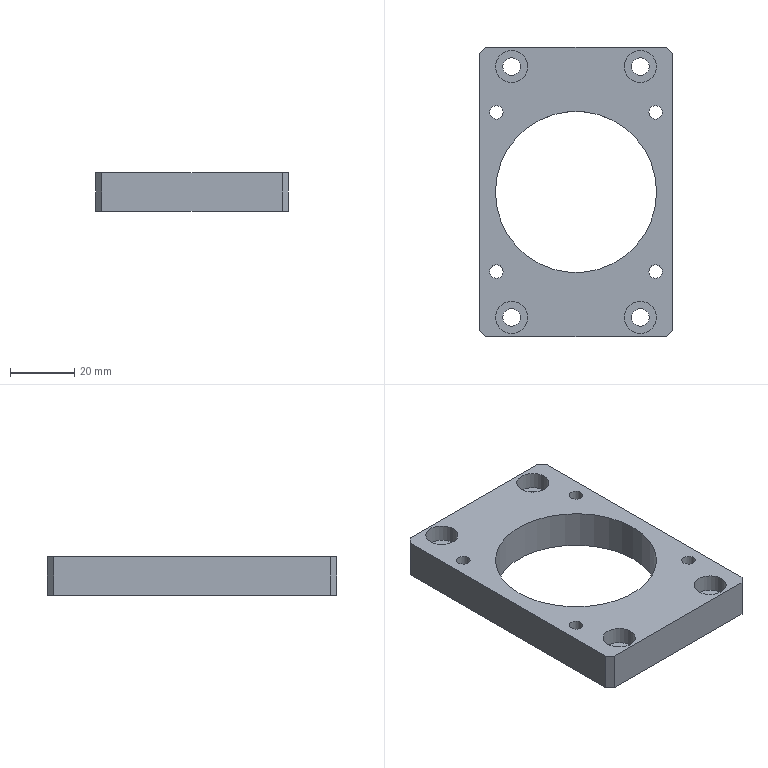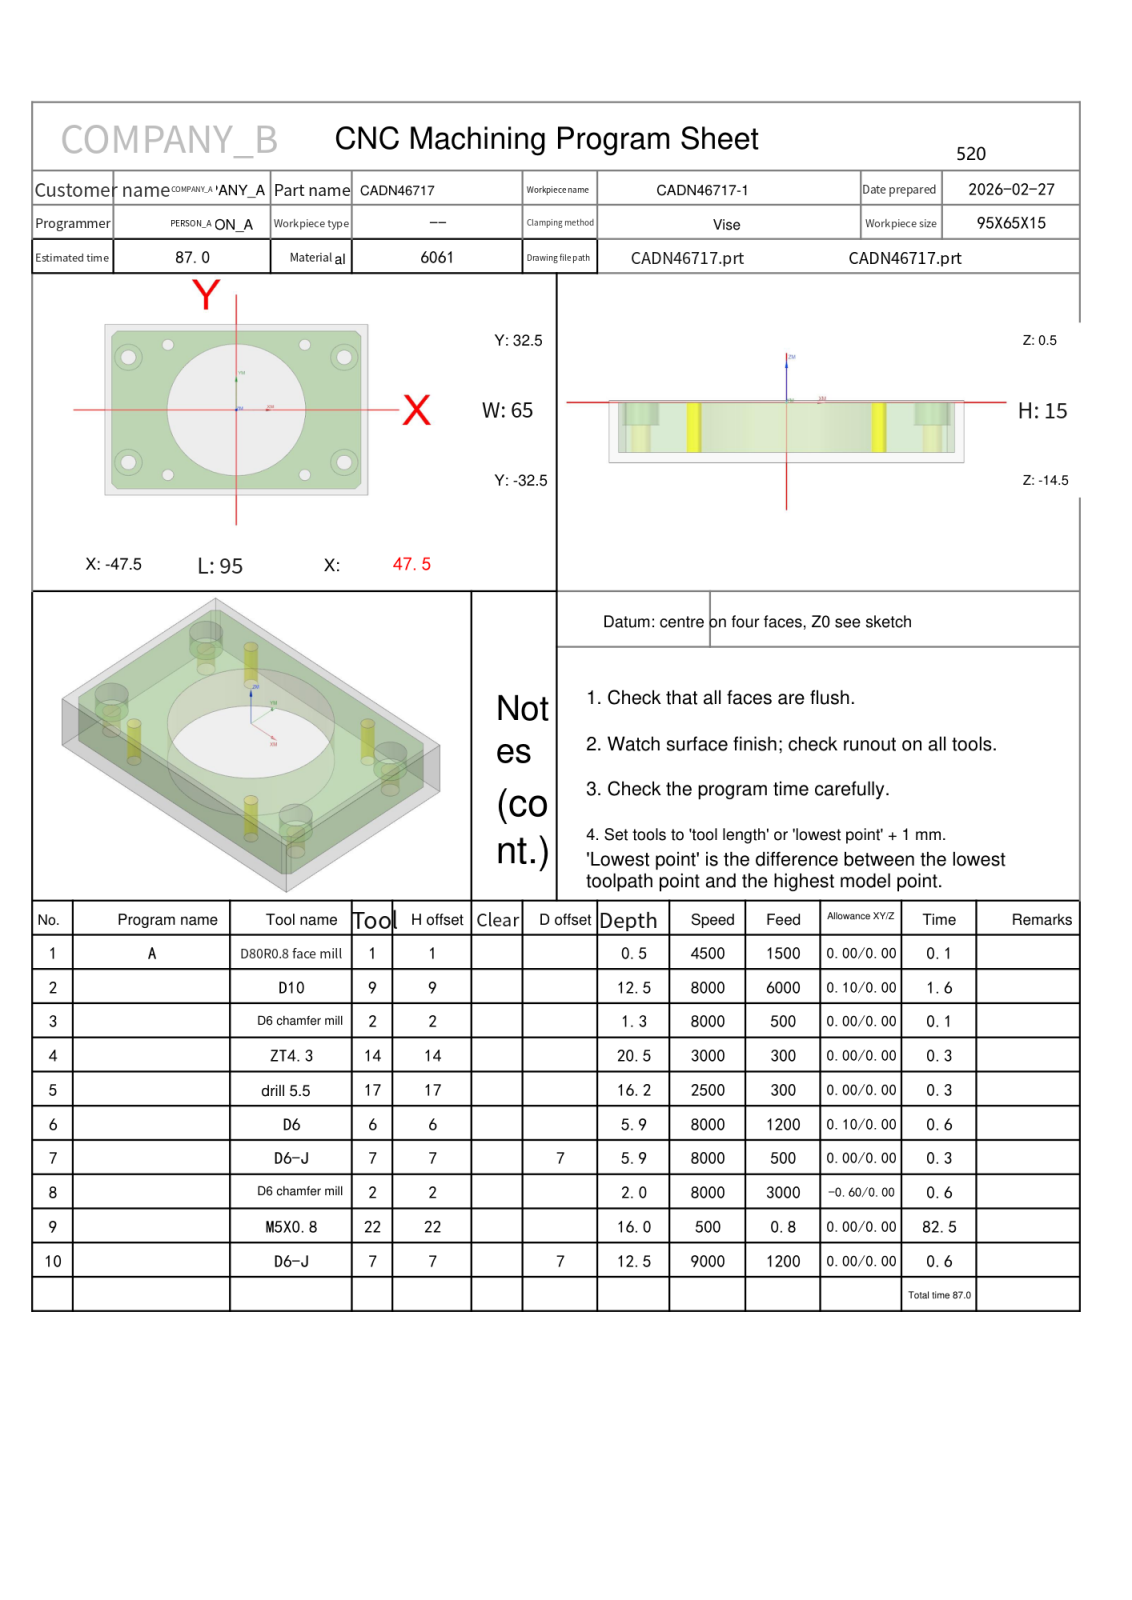NC program | NX | posted by the shop | part box 60 x 90 x 12 mm
Whole program:
%
O0001
(Machine time: 166.41 MIN)
(===Total Tool:8===)
(T1=D80R0.8 face mill D=80.  R=0.8  D-  H01 Z=-0.   )
(T9=D10     D=10.  R=0.   D-  H09 Z=-12.  )
(T2=D6 chamfer mill   D=6.   R=0.   D-  H02 Z=-1.5  )
(T14=ZT4.3  D=4.3  DR_a=118 D-  H14 Z=-20.  )
(T17=drill 5.5  D=5.5  DR_a=118 D-  H17 Z=-15.65)
(T6=D6      D=6.   R=0.   D-  H06 Z=-5.4  )
(T7=D6-J    D=6.   R=0.   D7  H07 Z=-12.  )
(T22=M5X0.8 D=4.2  DR_a=180 D-  H22 Z=-15.5 )
G80 G90 G17 G49 G40
G91 G28 Z0
M01
N1 T01 M06
(D80R0.8 face mill  D=80. R=0.8 H=01 ce=0.00 di=0.00)
G00 G90 G54 X-90. Y0.0 M03 S4500
G43 H01 Z50.
M08
Z2.
G01 Z0.0 F1500.
X-85.
X85.
X90.
Z2.
G00 Z50.
G91 G28 Z0.0
M05
M09
G91 G28 Z0.0
M01
N2 T09 M06
(D10  D=10. R=0. H=09 ce=0.10 di=0.00)
G00 G90 G54 X0.0 Y35.1 M03 S8000
G43 H09 Z50.
M08
Z.5
G01 X43. Z.397 F6000.
G02 X46.606 Y33.606 Z.388 I0.0 J-5.1
G01 X48.606 Y31.606 Z.381
G02 X50.1 Y28. Z.372 I-3.606 J-3.606
G01 Y-28. Z.238
G02 X48.606 Y-31.606 Z.228 I-5.1 J0.0
G01 X46.606 Y-33.606 Z.222
G02 X43. Y-35.1 Z.212 I-3.606 J3.606
G01 X-43. Z.007
G02 X-46.606 Y-33.606 Z-.003 I0.0 J5.1
G01 X-48.606 Y-31.606 Z-.01
G02 X-50.1 Y-28. Z-.019 I3.606 J3.606
G01 Y28. Z-.153
G02 X-48.606 Y31.606 Z-.162 I5.1 J0.0
G01 X-46.606 Y33.606 Z-.169
G02 X-43. Y35.1 Z-.179 I3.606 J-3.606
G01 X43. Z-.384
G02 X46.606 Y33.606 Z-.393 I0.0 J-5.1
G01 X48.606 Y31.606 Z-.4
G02 X50.1 Y28. Z-.41 I-3.606 J-3.606
G01 Y-28. Z-.543
G02 X48.606 Y-31.606 Z-.553 I-5.1 J0.0
G01 X46.606 Y-33.606 Z-.56
G02 X43. Y-35.1 Z-.569 I-3.606 J3.606
G01 X-43. Z-.774
G02 X-46.606 Y-33.606 Z-.784 I0.0 J5.1
G01 X-48.606 Y-31.606 Z-.791
G02 X-50.1 Y-28. Z-.8 I3.606 J3.606
G01 Y28. Z-.934
G02 X-48.606 Y31.606 Z-.944 I5.1 J0.0
G01 X-46.606 Y33.606 Z-.95
G02 X-43. Y35.1 Z-.96 I3.606 J-3.606
G01 X43. Z-1.165
G02 X46.606 Y33.606 Z-1.175 I0.0 J-5.1
G01 X48.606 Y31.606 Z-1.181
G02 X50.1 Y28. Z-1.191 I-3.606 J-3.606
G01 Y-28. Z-1.325
G02 X48.606 Y-31.606 Z-1.334 I-5.1 J0.0
G01 X46.606 Y-33.606 Z-1.341
G02 X43. Y-35.1 Z-1.351 I-3.606 J3.606
G01 X-43. Z-1.556
G02 X-46.606 Y-33.606 Z-1.565 I0.0 J5.1
G01 X-48.606 Y-31.606 Z-1.572
G02 X-50.1 Y-28. Z-1.582 I3.606 J3.606
G01 Y28. Z-1.715
G02 X-48.606 Y31.606 Z-1.725 I5.1 J0.0
G01 X-46.606 Y33.606 Z-1.732
G02 X-43. Y35.1 Z-1.741 I3.606 J-3.606
G01 X43. Z-1.946
G02 X46.606 Y33.606 Z-1.956 I0.0 J-5.1
G01 X48.606 Y31.606 Z-1.963
G02 X50.1 Y28. Z-1.972 I-3.606 J-3.606
G01 Y-28. Z-2.106
G02 X48.606 Y-31.606 Z-2.115 I-5.1 J0.0
G01 X46.606 Y-33.606 Z-2.122
G02 X43. Y-35.1 Z-2.132 I-3.606 J3.606
G01 X-43. Z-2.337
G02 X-46.606 Y-33.606 Z-2.347 I0.0 J5.1
G01 X-48.606 Y-31.606 Z-2.353
G02 X-50.1 Y-28. Z-2.363 I3.606 J3.606
G01 Y28. Z-2.497
G02 X-48.606 Y31.606 Z-2.506 I5.1 J0.0
G01 X-46.606 Y33.606 Z-2.513
G02 X-43. Y35.1 Z-2.522 I3.606 J-3.606
G01 X43. Z-2.728
G02 X46.606 Y33.606 Z-2.737 I0.0 J-5.1
G01 X48.606 Y31.606 Z-2.744
G02 X50.1 Y28. Z-2.753 I-3.606 J-3.606
G01 Y-28. Z-2.887
G02 X48.606 Y-31.606 Z-2.897 I-5.1 J0.0
G01 X46.606 Y-33.606 Z-2.903
G02 X43. Y-35.1 Z-2.913 I-3.606 J3.606
G01 X-43. Z-3.118
G02 X-46.606 Y-33.606 Z-3.128 I0.0 J5.1
G01 X-48.606 Y-31.606 Z-3.135
G02 X-50.1 Y-28. Z-3.144 I3.606 J3.606
G01 Y28. Z-3.278
G02 X-48.606 Y31.606 Z-3.287 I5.1 J0.0
G01 X-46.606 Y33.606 Z-3.294
G02 X-43. Y35.1 Z-3.304 I3.606 J-3.606
G01 X43. Z-3.509
G02 X46.606 Y33.606 Z-3.518 I0.0 J-5.1
G01 X48.606 Y31.606 Z-3.525
G02 X50.1 Y28. Z-3.535 I-3.606 J-3.606
G01 Y-28. Z-3.668
G02 X48.606 Y-31.606 Z-3.678 I-5.1 J0.0
G01 X46.606 Y-33.606 Z-3.685
G02 X43. Y-35.1 Z-3.694 I-3.606 J3.606
G01 X-43. Z-3.899
G02 X-46.606 Y-33.606 Z-3.909 I0.0 J5.1
G01 X-48.606 Y-31.606 Z-3.916
G02 X-50.1 Y-28. Z-3.925 I3.606 J3.606
G01 Y28. Z-4.059
G02 X-48.606 Y31.606 Z-4.069 I5.1 J0.0
G01 X-46.606 Y33.606 Z-4.075
G02 X-43. Y35.1 Z-4.085 I3.606 J-3.606
G01 X43. Z-4.29
G02 X46.606 Y33.606 Z-4.3 I0.0 J-5.1
G01 X48.606 Y31.606 Z-4.306
G02 X50.1 Y28. Z-4.316 I-3.606 J-3.606
G01 Y-28. Z-4.45
G02 X48.606 Y-31.606 Z-4.459 I-5.1 J0.0
G01 X46.606 Y-33.606 Z-4.466
G02 X43. Y-35.1 Z-4.476 I-3.606 J3.606
G01 X-43. Z-4.681
G02 X-46.606 Y-33.606 Z-4.69 I0.0 J5.1
G01 X-48.606 Y-31.606 Z-4.697
G02 X-50.1 Y-28. Z-4.707 I3.606 J3.606
G01 Y28. Z-4.84
G02 X-48.606 Y31.606 Z-4.85 I5.1 J0.0
G01 X-46.606 Y33.606 Z-4.857
G02 X-43. Y35.1 Z-4.866 I3.606 J-3.606
G01 X43. Z-5.071
G02 X46.606 Y33.606 Z-5.081 I0.0 J-5.1
G01 X48.606 Y31.606 Z-5.088
G02 X50.1 Y28. Z-5.097 I-3.606 J-3.606
G01 Y-28. Z-5.231
G02 X48.606 Y-31.606 Z-5.24 I-5.1 J0.0
G01 X46.606 Y-33.606 Z-5.247
G02 X43. Y-35.1 Z-5.257 I-3.606 J3.606
G01 X-43. Z-5.462
G02 X-46.606 Y-33.606 Z-5.472 I0.0 J5.1
G01 X-48.606 Y-31.606 Z-5.478
G02 X-50.1 Y-28. Z-5.488 I3.606 J3.606
G01 Y28. Z-5.622
G02 X-48.606 Y31.606 Z-5.631 I5.1 J0.0
G01 X-46.606 Y33.606 Z-5.638
G02 X-43. Y35.1 Z-5.647 I3.606 J-3.606
G01 X43. Z-5.853
G02 X46.606 Y33.606 Z-5.862 I0.0 J-5.1
G01 X48.606 Y31.606 Z-5.869
G02 X50.1 Y28. Z-5.878 I-3.606 J-3.606
G01 Y-28. Z-6.012
G02 X48.606 Y-31.606 Z-6.022 I-5.1 J0.0
G01 X46.606 Y-33.606 Z-6.028
G02 X43. Y-35.1 Z-6.038 I-3.606 J3.606
G01 X-43. Z-6.243
G02 X-46.606 Y-33.606 Z-6.253 I0.0 J5.1
G01 X-48.606 Y-31.606 Z-6.26
G02 X-50.1 Y-28. Z-6.269 I3.606 J3.606
G01 Y28. Z-6.403
G02 X-48.606 Y31.606 Z-6.412 I5.1 J0.0
G01 X-46.606 Y33.606 Z-6.419
G02 X-43. Y35.1 Z-6.429 I3.606 J-3.606
G01 X43. Z-6.634
G02 X46.606 Y33.606 Z-6.643 I0.0 J-5.1
G01 X48.606 Y31.606 Z-6.65
G02 X50.1 Y28. Z-6.66 I-3.606 J-3.606
G01 Y-28. Z-6.793
G02 X48.606 Y-31.606 Z-6.803 I-5.1 J0.0
G01 X46.606 Y-33.606 Z-6.81
G02 X43. Y-35.1 Z-6.819 I-3.606 J3.606
G01 X-43. Z-7.024
G02 X-46.606 Y-33.606 Z-7.034 I0.0 J5.1
G01 X-48.606 Y-31.606 Z-7.041
G02 X-50.1 Y-28. Z-7.05 I3.606 J3.606
G01 Y28. Z-7.184
G02 X-48.606 Y31.606 Z-7.194 I5.1 J0.0
G01 X-46.606 Y33.606 Z-7.2
G02 X-43. Y35.1 Z-7.21 I3.606 J-3.606
G01 X43. Z-7.415
G02 X46.606 Y33.606 Z-7.425 I0.0 J-5.1
G01 X48.606 Y31.606 Z-7.431
G02 X50.1 Y28. Z-7.441 I-3.606 J-3.606
G01 Y-28. Z-7.575
G02 X48.606 Y-31.606 Z-7.584 I-5.1 J0.0
G01 X46.606 Y-33.606 Z-7.591
G02 X43. Y-35.1 Z-7.601 I-3.606 J3.606
G01 X-43. Z-7.806
G02 X-46.606 Y-33.606 Z-7.815 I0.0 J5.1
G01 X-48.606 Y-31.606 Z-7.822
G02 X-50.1 Y-28. Z-7.832 I3.606 J3.606
G01 Y28. Z-7.965
G02 X-48.606 Y31.606 Z-7.975 I5.1 J0.0
G01 X-46.606 Y33.606 Z-7.982
G02 X-43. Y35.1 Z-7.991 I3.606 J-3.606
G01 X43. Z-8.196
G02 X46.606 Y33.606 Z-8.206 I0.0 J-5.1
G01 X48.606 Y31.606 Z-8.213
G02 X50.1 Y28. Z-8.222 I-3.606 J-3.606
G01 Y-28. Z-8.356
G02 X48.606 Y-31.606 Z-8.365 I-5.1 J0.0
G01 X46.606 Y-33.606 Z-8.372
G02 X43. Y-35.1 Z-8.382 I-3.606 J3.606
G01 X-43. Z-8.587
G02 X-46.606 Y-33.606 Z-8.597 I0.0 J5.1
G01 X-48.606 Y-31.606 Z-8.603
G02 X-50.1 Y-28. Z-8.613 I3.606 J3.606
G01 Y28. Z-8.747
G02 X-48.606 Y31.606 Z-8.756 I5.1 J0.0
G01 X-46.606 Y33.606 Z-8.763
G02 X-43. Y35.1 Z-8.772 I3.606 J-3.606
G01 X43. Z-8.978
G02 X46.606 Y33.606 Z-8.987 I0.0 J-5.1
G01 X48.606 Y31.606 Z-8.994
G02 X50.1 Y28. Z-9.003 I-3.606 J-3.606
G01 Y-28. Z-9.137
G02 X48.606 Y-31.606 Z-9.147 I-5.1 J0.0
G01 X46.606 Y-33.606 Z-9.153
G02 X43. Y-35.1 Z-9.163 I-3.606 J3.606
G01 X-43. Z-9.368
G02 X-46.606 Y-33.606 Z-9.378 I0.0 J5.1
G01 X-48.606 Y-31.606 Z-9.385
G02 X-50.1 Y-28. Z-9.394 I3.606 J3.606
G01 Y28. Z-9.528
G02 X-48.606 Y31.606 Z-9.537 I5.1 J0.0
G01 X-46.606 Y33.606 Z-9.544
G02 X-43. Y35.1 Z-9.554 I3.606 J-3.606
G01 X43. Z-9.759
G02 X46.606 Y33.606 Z-9.768 I0.0 J-5.1
G01 X48.606 Y31.606 Z-9.775
G02 X50.1 Y28. Z-9.785 I-3.606 J-3.606
G01 Y-28. Z-9.918
G02 X48.606 Y-31.606 Z-9.928 I-5.1 J0.0
G01 X46.606 Y-33.606 Z-9.935
G02 X43. Y-35.1 Z-9.944 I-3.606 J3.606
G01 X-43. Z-10.149
G02 X-46.606 Y-33.606 Z-10.159 I0.0 J5.1
G01 X-48.606 Y-31.606 Z-10.166
G02 X-50.1 Y-28. Z-10.175 I3.606 J3.606
G01 Y28. Z-10.309
G02 X-48.606 Y31.606 Z-10.319 I5.1 J0.0
G01 X-46.606 Y33.606 Z-10.325
G02 X-43. Y35.1 Z-10.335 I3.606 J-3.606
G01 X43. Z-10.54
G02 X46.606 Y33.606 Z-10.55 I0.0 J-5.1
G01 X48.606 Y31.606 Z-10.556
G02 X50.1 Y28. Z-10.566 I-3.606 J-3.606
G01 Y-28. Z-10.7
G02 X48.606 Y-31.606 Z-10.709 I-5.1 J0.0
G01 X46.606 Y-33.606 Z-10.716
G02 X43. Y-35.1 Z-10.726 I-3.606 J3.606
G01 X-43. Z-10.931
G02 X-46.606 Y-33.606 Z-10.94 I0.0 J5.1
G01 X-48.606 Y-31.606 Z-10.947
G02 X-50.1 Y-28. Z-10.957 I3.606 J3.606
G01 Y28. Z-11.09
G02 X-48.606 Y31.606 Z-11.1 I5.1 J0.0
G01 X-46.606 Y33.606 Z-11.107
G02 X-43. Y35.1 Z-11.116 I3.606 J-3.606
G01 X43. Z-11.321
G02 X46.606 Y33.606 Z-11.331 I0.0 J-5.1
G01 X48.606 Y31.606 Z-11.338
G02 X50.1 Y28. Z-11.347 I-3.606 J-3.606
G01 Y-28. Z-11.481
G02 X48.606 Y-31.606 Z-11.49 I-5.1 J0.0
G01 X46.606 Y-33.606 Z-11.497
G02 X43. Y-35.1 Z-11.507 I-3.606 J3.606
G01 X-43. Z-11.712
G02 X-46.606 Y-33.606 Z-11.722 I0.0 J5.1
G01 X-48.606 Y-31.606 Z-11.728
G02 X-50.1 Y-28. Z-11.738 I3.606 J3.606
G01 Y28. Z-11.872
G02 X-48.606 Y31.606 Z-11.881 I5.1 J0.0
G01 X-46.606 Y33.606 Z-11.888
G02 X-43. Y35.1 Z-11.897 I3.606 J-3.606
G01 X0.0 Z-12.
X43.
G02 X46.606 Y33.606 I0.0 J-5.1
G01 X48.606 Y31.606
G02 X50.1 Y28. I-3.606 J-3.606
G01 Y-28.
G02 X48.606 Y-31.606 I-5.1 J0.0
G01 X46.606 Y-33.606
G02 X43. Y-35.1 I-3.606 J3.606
G01 X-43.
G02 X-46.606 Y-33.606 I0.0 J5.1
G01 X-48.606 Y-31.606
G02 X-50.1 Y-28. I3.606 J3.606
G01 Y28.
G02 X-48.606 Y31.606 I5.1 J0.0
G01 X-46.606 Y33.606
G02 X-43. Y35.1 I3.606 J-3.606
G01 X0.0
X.5
Z-11.
G00 Z50.
G00 G90 X-16.295 Y-11.511 M03 S8000
Z50.
Z1.
G01 X-16.034 Y-11.92 Z.975 F4000.
X-14.128 Y-14.128 Z.822
X-11.92 Y-16.034 Z.669
X-9.459 Y-17.599 Z.516
X-6.796 Y-18.789 Z.363
X-3.988 Y-19.578 Z.21
X-1.094 Y-19.95 Z.057
X0.0 Z0.0
G03 X19.95 Y0.0 Z-.149 I0.0 J19.95
X0.0 Y19.95 Z-.298 I-19.95 J0.0
X-19.95 Y0.0 Z-.446 I0.0 J-19.95
X0.0 Y-19.95 Z-.595 I19.95 J0.0
X19.95 Y0.0 Z-.744 I0.0 J19.95
X0.0 Y19.95 Z-.893 I-19.95 J0.0
X-19.95 Y0.0 Z-1.041 I0.0 J-19.95
X0.0 Y-19.95 Z-1.19 I19.95 J0.0
X19.95 Y0.0 Z-1.339 I0.0 J19.95
X0.0 Y19.95 Z-1.488 I-19.95 J0.0
X-19.95 Y0.0 Z-1.636 I0.0 J-19.95
X0.0 Y-19.95 Z-1.785 I19.95 J0.0
X19.95 Y0.0 Z-1.934 I0.0 J19.95
X0.0 Y19.95 Z-2.083 I-19.95 J0.0
X-19.95 Y0.0 Z-2.231 I0.0 J-19.95
X0.0 Y-19.95 Z-2.38 I19.95 J0.0
X19.95 Y0.0 Z-2.529 I0.0 J19.95
X0.0 Y19.95 Z-2.678 I-19.95 J0.0
X-19.95 Y0.0 Z-2.826 I0.0 J-19.95
X0.0 Y-19.95 Z-2.975 I19.95 J0.0
X19.95 Y0.0 Z-3.124 I0.0 J19.95
X0.0 Y19.95 Z-3.273 I-19.95 J0.0
X-19.95 Y0.0 Z-3.421 I0.0 J-19.95
X0.0 Y-19.95 Z-3.57 I19.95 J0.0
X19.95 Y0.0 Z-3.719 I0.0 J19.95
X0.0 Y19.95 Z-3.868 I-19.95 J0.0
X-19.95 Y0.0 Z-4.016 I0.0 J-19.95
X0.0 Y-19.95 Z-4.165 I19.95 J0.0
X19.95 Y0.0 Z-4.314 I0.0 J19.95
X0.0 Y19.95 Z-4.463 I-19.95 J0.0
X-19.95 Y0.0 Z-4.611 I0.0 J-19.95
X0.0 Y-19.95 Z-4.76 I19.95 J0.0
X19.95 Y0.0 Z-4.909 I0.0 J19.95
X0.0 Y19.95 Z-5.058 I-19.95 J0.0
X-19.95 Y0.0 Z-5.206 I0.0 J-19.95
X0.0 Y-19.95 Z-5.355 I19.95 J0.0
X19.95 Y0.0 Z-5.504 I0.0 J19.95
X0.0 Y19.95 Z-5.653 I-19.95 J0.0
X-19.95 Y0.0 Z-5.801 I0.0 J-19.95
X0.0 Y-19.95 Z-5.95 I19.95 J0.0
X19.95 Y0.0 Z-6.099 I0.0 J19.95
X0.0 Y19.95 Z-6.248 I-19.95 J0.0
X-19.95 Y0.0 Z-6.396 I0.0 J-19.95
X0.0 Y-19.95 Z-6.545 I19.95 J0.0
X19.95 Y0.0 Z-6.694 I0.0 J19.95
X0.0 Y19.95 Z-6.843 I-19.95 J0.0
X-19.95 Y0.0 Z-6.991 I0.0 J-19.95
X0.0 Y-19.95 Z-7.14 I19.95 J0.0
X19.95 Y0.0 Z-7.289 I0.0 J19.95
X0.0 Y19.95 Z-7.438 I-19.95 J0.0
X-19.95 Y0.0 Z-7.586 I0.0 J-19.95
X0.0 Y-19.95 Z-7.735 I19.95 J0.0
X19.95 Y0.0 Z-7.884 I0.0 J19.95
X0.0 Y19.95 Z-8.033 I-19.95 J0.0
X-19.95 Y0.0 Z-8.181 I0.0 J-19.95
X0.0 Y-19.95 Z-8.33 I19.95 J0.0
X19.95 Y0.0 Z-8.479 I0.0 J19.95
X0.0 Y19.95 Z-8.628 I-19.95 J0.0
X-19.95 Y0.0 Z-8.776 I0.0 J-19.95
X0.0 Y-19.95 Z-8.925 I19.95 J0.0
X19.95 Y0.0 Z-9.074 I0.0 J19.95
X0.0 Y19.95 Z-9.223 I-19.95 J0.0
X-19.95 Y0.0 Z-9.371 I0.0 J-19.95
X0.0 Y-19.95 Z-9.52 I19.95 J0.0
X19.95 Y0.0 Z-9.669 I0.0 J19.95
X0.0 Y19.95 Z-9.818 I-19.95 J0.0
X-19.95 Y0.0 Z-9.966 I0.0 J-19.95
X0.0 Y-19.95 Z-10.115 I19.95 J0.0
X19.95 Y0.0 Z-10.264 I0.0 J19.95
X0.0 Y19.95 Z-10.413 I-19.95 J0.0
X-19.95 Y0.0 Z-10.561 I0.0 J-19.95
X0.0 Y-19.95 Z-10.71 I19.95 J0.0
X19.95 Y0.0 Z-10.859 I0.0 J19.95
X0.0 Y19.95 Z-11.008 I-19.95 J0.0
X-19.95 Y0.0 Z-11.156 I0.0 J-19.95
X0.0 Y-19.95 Z-11.305 I19.95 J0.0
X19.95 Y0.0 Z-11.454 I0.0 J19.95
X0.0 Y19.95 Z-11.603 I-19.95 J0.0
X-19.95 Y0.0 Z-11.751 I0.0 J-19.95
X0.0 Y-19.95 Z-11.9 I19.95 J0.0
X19.95 Y0.0 I0.0 J19.95
X0.0 Y19.95 I-19.95 J0.0
X-19.95 Y0.0 I0.0 J-19.95
X0.0 Y-19.95 I19.95 J0.0
X.4 Y-19.946 I0.0 J19.95
G01 Z-10.9
G00 Z50.
G91 G28 Z0.0
M05
M09
G91 G28 Z0.0
M01
N3 T02 M06
(D6 chamfer mill  D=6. R=0. H=02 ce=0.00 di=0.10)
G00 G90 G54 X24.749 Y-24.749 M03 S8000
G43 H02 Z50.
M08
G98 G81 X24.749 Y-24.749 Z-.8 R1. F500.
X39. Y-20.
Y20.
X24.749 Y24.749
X-24.749
X-39. Y20.
Y-20.
X-24.749 Y-24.749
G80
G00 Z50.
G91 G28 Z0.0
M05
M09
G91 G28 Z0.0
M01
N4 T14 M06
(ZT4.3 D=4.3 DR_a=118 H=14)
G00 G90 G54 X24.749 Y-24.749 M03 S3000
G43 H14 Z50.
M08
G98 G83 X24.749 Y-24.749 Z-20. R1. F300. Q3.
X-24.749
Y24.749
X24.749
G80
G00 Z50.
G91 G28 Z0.0
M05
M09
G91 G28 Z0.0
M01
N5 T17 M06
(drill 5.5 D=5.5 DR_a=118 H=17)
G00 G90 G54 X39. Y-20. M03 S2500
G43 H17 Z50.
M08
G98 G83 X39. Y-20. Z-15.652 R1. F300. Q2.
Y20.
X-39.
Y-20.
G80
G00 Z50.
G91 G28 Z0.0
M05
M09
G91 G28 Z0.0
M01
N6 T06 M06
(D6  D=6. R=0. H=06 ce=0.10 di=0.00)
G00 G90 G54 X39. Y-20. M03 S8000
G43 H06 Z50.
M08
Z.5
G03 X38.05 Y-20.95 I0.0 J-.95 F1200.
X39. Y-21.9 I.95 J0.0
X39. Y-21.9 Z0.0 I0.0 J1.9
X39. Y-21.9 Z-.5 I0.0 J1.9
X39. Y-21.9 Z-1. I0.0 J1.9
X39. Y-21.9 Z-1.5 I0.0 J1.9
X39. Y-21.9 Z-2. I0.0 J1.9
X39. Y-21.9 Z-2.5 I0.0 J1.9
X39. Y-21.9 Z-3. I0.0 J1.9
X39. Y-21.9 Z-3.5 I0.0 J1.9
X39. Y-21.9 Z-4. I0.0 J1.9
X39. Y-21.9 Z-4.5 I0.0 J1.9
X39. Y-21.9 Z-5. I0.0 J1.9
X37.193 Y-20.587 Z-5.4 I0.0 J1.9
X39. Y-21.9 I1.807 J.587
X40.9 Y-20. I0.0 J1.9
X39. Y-18.1 I-1.9 J0.0
X37.1 Y-20. I0.0 J-1.9
X37.193 Y-20.587 I1.9 J0.0
X38.096 Y-21.244 I.904 J.294
X39.046 Y-20.294 I0.0 J.95
X39. Y-20. I-.95 J0.0
G00 Z50.
Y20.
Z.5
G03 X38.05 Y19.05 I0.0 J-.95
X39. Y18.1 I.95 J0.0
X39. Y18.1 Z0.0 I0.0 J1.9
X39. Y18.1 Z-.5 I0.0 J1.9
X39. Y18.1 Z-1. I0.0 J1.9
X39. Y18.1 Z-1.5 I0.0 J1.9
X39. Y18.1 Z-2. I0.0 J1.9
X39. Y18.1 Z-2.5 I0.0 J1.9
X39. Y18.1 Z-3. I0.0 J1.9
X39. Y18.1 Z-3.5 I0.0 J1.9
X39. Y18.1 Z-4. I0.0 J1.9
X39. Y18.1 Z-4.5 I0.0 J1.9
X39. Y18.1 Z-5. I0.0 J1.9
X37.193 Y19.413 Z-5.4 I0.0 J1.9
X39. Y18.1 I1.807 J.587
X40.9 Y20. I0.0 J1.9
X39. Y21.9 I-1.9 J0.0
X37.1 Y20. I0.0 J-1.9
X37.193 Y19.413 I1.9 J0.0
X38.096 Y18.756 I.904 J.294
X39.046 Y19.706 I0.0 J.95
X39. Y20. I-.95 J0.0
G00 Z50.
X-39.
Z.5
G03 X-39.95 Y19.05 I0.0 J-.95
X-39. Y18.1 I.95 J0.0
X-39. Y18.1 Z0.0 I0.0 J1.9
X-39. Y18.1 Z-.5 I0.0 J1.9
X-39. Y18.1 Z-1. I0.0 J1.9
X-39. Y18.1 Z-1.5 I0.0 J1.9
X-39. Y18.1 Z-2. I0.0 J1.9
X-39. Y18.1 Z-2.5 I0.0 J1.9
X-39. Y18.1 Z-3. I0.0 J1.9
X-39. Y18.1 Z-3.5 I0.0 J1.9
X-39. Y18.1 Z-4. I0.0 J1.9
X-39. Y18.1 Z-4.5 I0.0 J1.9
X-39. Y18.1 Z-5. I0.0 J1.9
X-40.807 Y19.413 Z-5.4 I0.0 J1.9
X-39. Y18.1 I1.807 J.587
X-37.1 Y20. I0.0 J1.9
X-39. Y21.9 I-1.9 J0.0
X-40.9 Y20. I0.0 J-1.9
X-40.807 Y19.413 I1.9 J0.0
X-39.904 Y18.756 I.904 J.294
X-38.954 Y19.706 I0.0 J.95
X-39. Y20. I-.95 J0.0
G00 Z50.
Y-20.
Z.5
G03 X-39.95 Y-20.95 I0.0 J-.95
X-39. Y-21.9 I.95 J0.0
X-39. Y-21.9 Z0.0 I0.0 J1.9
X-39. Y-21.9 Z-.5 I0.0 J1.9
X-39. Y-21.9 Z-1. I0.0 J1.9
X-39. Y-21.9 Z-1.5 I0.0 J1.9
X-39. Y-21.9 Z-2. I0.0 J1.9
X-39. Y-21.9 Z-2.5 I0.0 J1.9
X-39. Y-21.9 Z-3. I0.0 J1.9
X-39. Y-21.9 Z-3.5 I0.0 J1.9
X-39. Y-21.9 Z-4. I0.0 J1.9
X-39. Y-21.9 Z-4.5 I0.0 J1.9
X-39. Y-21.9 Z-5. I0.0 J1.9
X-40.807 Y-20.587 Z-5.4 I0.0 J1.9
X-39. Y-21.9 I1.807 J.587
X-37.1 Y-20. I0.0 J1.9
X-39. Y-18.1 I-1.9 J0.0
X-40.9 Y-20. I0.0 J-1.9
X-40.807 Y-20.587 I1.9 J0.0
X-39.904 Y-21.244 I.904 J.294
X-38.954 Y-20.294 I0.0 J.95
X-39. Y-20. I-.95 J0.0
G00 Z50.
G91 G28 Z0.0
M05
M09
G91 G28 Z0.0
M01
N7 T07 M06
(D6-J  D=6. R=0. H=07 ce=0.00 di=0.00)
G00 G90 G54 X39. Y-20. M03 S8000
G43 H07 Z50.
M08
Z0.0
G41 D07
G01 X38.804 Y-20.04 F500.
G03 X38.01 Y-21.01 I.196 J-.97
X39. Y-22. I.99 J0.0
X39. Y-22. Z-5. I0.0 J2.
X39.964 Y-21.753 Z-5.4 I0.0 J2.
X41. Y-20. I-.964 J1.753
X39. Y-18. I-2. J0.0
X37. Y-20. I0.0 J-2.
X39. Y-22. I2. J0.0
X39.964 Y-21.753 I0.0 J2.
X40.477 Y-20.885 I-.477 J.868
X39.487 Y-19.895 I-.99 J0.0
X39.191 Y-19.94 I0.0 J-.99
G01 G40 X39. Y-20.
G00 Z50.
Y20.
Z0.0
G41 D07
G01 X38.804 Y19.96
G03 X38.01 Y18.99 I.196 J-.97
X39. Y18. I.99 J0.0
X39. Y18. Z-5. I0.0 J2.
X39.964 Y18.247 Z-5.4 I0.0 J2.
X41. Y20. I-.964 J1.753
X39. Y22. I-2. J0.0
X37. Y20. I0.0 J-2.
X39. Y18. I2. J0.0
X39.964 Y18.247 I0.0 J2.
X40.477 Y19.115 I-.477 J.868
X39.487 Y20.105 I-.99 J0.0
X39.191 Y20.06 I0.0 J-.99
G01 G40 X39. Y20.
G00 Z50.
X-39.
Z0.0
G41 D07
G01 X-39.196 Y19.96
G03 X-39.99 Y18.99 I.196 J-.97
X-39. Y18. I.99 J0.0
X-39. Y18. Z-5. I0.0 J2.
X-38.036 Y18.247 Z-5.4 I0.0 J2.
X-37. Y20. I-.964 J1.753
X-39. Y22. I-2. J0.0
X-41. Y20. I0.0 J-2.
X-39. Y18. I2. J0.0
X-38.036 Y18.247 I0.0 J2.
X-37.523 Y19.115 I-.477 J.868
X-38.513 Y20.105 I-.99 J0.0
X-38.809 Y20.06 I0.0 J-.99
G01 G40 X-39. Y20.
G00 Z50.
Y-20.
Z0.0
G41 D07
G01 X-39.196 Y-20.04
G03 X-39.99 Y-21.01 I.196 J-.97
X-39. Y-22. I.99 J0.0
X-39. Y-22. Z-5. I0.0 J2.
X-38.036 Y-21.753 Z-5.4 I0.0 J2.
X-37. Y-20. I-.964 J1.753
X-39. Y-18. I-2. J0.0
X-41. Y-20. I0.0 J-2.
X-39. Y-22. I2. J0.0
X-38.036 Y-21.753 I0.0 J2.
X-37.523 Y-20.885 I-.477 J.868
X-38.513 Y-19.895 I-.99 J0.0
X-38.809 Y-19.94 I0.0 J-.99
G01 G40 X-39. Y-20.
G00 Z50.
G91 G28 Z0.0
M05
M09
G91 G28 Z0.0
M01
N8 T02 M06
(D6 chamfer mill  D=6. R=0. H=02 ce=0.00 di=0.00)
G00 G90 G54 X-.25 Y32.128 M03 S8000
G43 H02 Z50.
M08
Z2.099
G01 Z-1.5 F3000.
G03 X-.33 Y31.828 I.52 J-.3
X-.03 Y31.308 I.6 J0.0
G01 X0.0 Y31.3
X43.
X43.254 Y31.275
X43.497 Y31.201
X43.722 Y31.081
X43.919 Y30.919
X45.919 Y28.919
X46.081 Y28.722
X46.201 Y28.497
X46.275 Y28.254
X46.3 Y28.
Y-28.
X46.275 Y-28.254
X46.201 Y-28.497
X46.081 Y-28.722
X45.919 Y-28.919
X43.919 Y-30.919
X43.722 Y-31.081
X43.497 Y-31.201
X43.254 Y-31.275
X43. Y-31.3
X-43.
X-43.254 Y-31.275
X-43.497 Y-31.201
X-43.722 Y-31.081
X-43.919 Y-30.919
X-45.919 Y-28.919
X-46.081 Y-28.722
X-46.201 Y-28.497
X-46.275 Y-28.254
X-46.3 Y-28.
Y28.
X-46.275 Y28.254
X-46.201 Y28.497
X-46.081 Y28.722
X-45.919 Y28.919
X-43.919 Y30.919
X-43.722 Y31.081
X-43.497 Y31.201
X-43.254 Y31.275
X-43. Y31.3
X0.0
X.03 Y31.308
G03 X.33 Y31.828 I-.3 J.52
X.25 Y32.128 I-.6 J0.0
G01 Z2.099
G00 Z6.
X.272 Y22.93
Z2.115
G01 Z-1.5
G03 X.345 Y23.215 I-.528 J.286
X.03 Y23.743 I-.6 J0.0
G01 X0.0 Y23.75
G03 X-23.75 Y0.0 I0.0 J-23.75
X0.0 Y-23.75 I23.75 J0.0
X23.75 Y0.0 I0.0 J23.75
X0.0 Y23.75 I-23.75 J0.0
G01 X-.03 Y23.743
G03 X-.345 Y23.215 I.286 J-.528
X-.272 Y22.93 I.6 J0.0
G01 Z2.115
G00 Z50.
G00 G90 X25.443 Y-24.656 M03 S8000
Z50.
Z-.5
G01 Z-1. F500.
X26.249 Y-24.549
G03 X24.749 Y-23.049 I-1.5 J0.0
X23.049 Y-24.749 I0.0 J-1.7
X24.749 Y-26.449 I1.7 J0.0
X26.449 Y-24.749 I0.0 J1.7
X24.749 Y-23.049 I-1.7 J0.0
X23.249 Y-24.549 I0.0 J-1.5
G01 X24.055 Y-24.656
Z-.5
G00 Z50.
X-24.055
Z-.5
G01 Z-1.
X-23.249 Y-24.549
G03 X-24.749 Y-23.049 I-1.5 J0.0
X-26.449 Y-24.749 I0.0 J-1.7
X-24.749 Y-26.449 I1.7 J0.0
X-23.049 Y-24.749 I0.0 J1.7
X-24.749 Y-23.049 I-1.7 J0.0
X-26.249 Y-24.549 I0.0 J-1.5
G01 X-25.443 Y-24.656
Z-.5
G00 Z50.
X-24.055 Y24.841
Z-.5
G01 Z-1.
X-23.249 Y24.949
G03 X-24.749 Y26.449 I-1.5 J0.0
X-26.449 Y24.749 I0.0 J-1.7
X-24.749 Y23.049 I1.7 J0.0
X-23.049 Y24.749 I0.0 J1.7
X-24.749 Y26.449 I-1.7 J0.0
X-26.249 Y24.949 I0.0 J-1.5
G01 X-25.443 Y24.841
Z-.5
G00 Z50.
X25.443
Z-.5
G01 Z-1.
X26.249 Y24.949
G03 X24.749 Y26.449 I-1.5 J0.0
X23.049 Y24.749 I0.0 J-1.7
X24.749 Y23.049 I1.7 J0.0
X26.449 Y24.749 I0.0 J1.7
X24.749 Y26.449 I-1.7 J0.0
X23.249 Y24.949 I0.0 J-1.5
G01 X24.055 Y24.841
Z-.5
G00 Z50.
G00 G90 X35.614 Y-17.346 M03 S8000
Z50.
Z2.5
G01 X35.606 Y-17.355 Z2.495 F800.
X35.356 Y-17.711 Z2.337
X35.196 Y-17.989 Z2.22
X35.012 Y-18.383 Z2.062
X34.87 Y-18.793 Z1.904
X34.769 Y-19.216 Z1.746
X34.712 Y-19.646 Z1.588
X34.698 Y-20.08 Z1.43
X34.728 Y-20.514 Z1.272
X34.801 Y-20.942 Z1.114
X34.918 Y-21.36 Z.956
X35.076 Y-21.765 Z.797
X35.273 Y-22.152 Z.639
X35.509 Y-22.516 Z.481
X35.781 Y-22.855 Z.323
X36.085 Y-23.165 Z.165
X36.419 Y-23.443 Z.007
X36.779 Y-23.686 Z-.151
X37.162 Y-23.891 Z-.309
X37.564 Y-24.056 Z-.467
X37.98 Y-24.18 Z-.625
X38.407 Y-24.262 Z-.783
X38.839 Y-24.3 Z-.942
X39. Z-1.
G03 X43.3 Y-20. I0.0 J4.3
X39. Y-15.7 I-4.3 J0.0
X34.7 Y-20. I0.0 J-4.3
X39. Y-24.3 I4.3 J0.0
X39.499 Y-24.271 I0.0 J4.3
G01 Z1.5
G00 Z50.
X35.614 Y22.654
Z2.5
G01 X35.606 Y22.645 Z2.495
X35.356 Y22.289 Z2.337
X35.196 Y22.011 Z2.22
X35.012 Y21.617 Z2.062
X34.87 Y21.207 Z1.904
X34.769 Y20.784 Z1.746
X34.712 Y20.354 Z1.588
X34.698 Y19.92 Z1.43
X34.728 Y19.486 Z1.272
X34.801 Y19.058 Z1.114
X34.918 Y18.64 Z.956
X35.076 Y18.235 Z.797
X35.273 Y17.849 Z.639
X35.509 Y17.484 Z.481
X35.781 Y17.145 Z.323
X36.085 Y16.835 Z.165
X36.419 Y16.557 Z.007
X36.779 Y16.314 Z-.151
X37.162 Y16.109 Z-.309
X37.564 Y15.944 Z-.467
X37.98 Y15.82 Z-.625
X38.407 Y15.738 Z-.783
X38.839 Y15.7 Z-.942
X39. Z-1.
G03 X43.3 Y20. I0.0 J4.3
X39. Y24.3 I-4.3 J0.0
X34.7 Y20. I0.0 J-4.3
X39. Y15.7 I4.3 J0.0
X39.499 Y15.729 I0.0 J4.3
G01 Z1.5
G00 Z50.
X-42.386 Y22.654
Z2.5
G01 X-42.394 Y22.645 Z2.495
X-42.644 Y22.289 Z2.337
X-42.804 Y22.011 Z2.22
X-42.988 Y21.617 Z2.062
X-43.13 Y21.207 Z1.904
X-43.231 Y20.784 Z1.746
X-43.288 Y20.354 Z1.588
X-43.302 Y19.92 Z1.43
X-43.272 Y19.486 Z1.272
X-43.199 Y19.058 Z1.114
X-43.082 Y18.64 Z.956
X-42.924 Y18.235 Z.797
X-42.727 Y17.849 Z.639
X-42.491 Y17.484 Z.481
X-42.219 Y17.145 Z.323
X-41.915 Y16.835 Z.165
X-41.581 Y16.557 Z.007
X-41.221 Y16.314 Z-.151
X-40.838 Y16.109 Z-.309
X-40.436 Y15.944 Z-.467
X-40.02 Y15.82 Z-.625
X-39.593 Y15.738 Z-.783
X-39.161 Y15.7 Z-.942
X-39. Z-1.
G03 X-34.7 Y20. I0.0 J4.3
X-39. Y24.3 I-4.3 J0.0
X-43.3 Y20. I0.0 J-4.3
X-39. Y15.7 I4.3 J0.0
X-38.501 Y15.729 I0.0 J4.3
G01 Z1.5
G00 Z50.
X-42.386 Y-17.346
Z2.5
G01 X-42.394 Y-17.355 Z2.495
X-42.644 Y-17.711 Z2.337
X-42.804 Y-17.989 Z2.22
X-42.988 Y-18.383 Z2.062
X-43.13 Y-18.793 Z1.904
X-43.231 Y-19.216 Z1.746
X-43.288 Y-19.646 Z1.588
X-43.302 Y-20.08 Z1.43
X-43.272 Y-20.514 Z1.272
X-43.199 Y-20.942 Z1.114
X-43.082 Y-21.36 Z.956
X-42.924 Y-21.765 Z.797
X-42.727 Y-22.152 Z.639
X-42.491 Y-22.516 Z.481
X-42.219 Y-22.855 Z.323
X-41.915 Y-23.165 Z.165
X-41.581 Y-23.443 Z.007
X-41.221 Y-23.686 Z-.151
X-40.838 Y-23.891 Z-.309
X-40.436 Y-24.056 Z-.467
X-40.02 Y-24.18 Z-.625
X-39.593 Y-24.262 Z-.783
X-39.161 Y-24.3 Z-.942
X-39. Z-1.
G03 X-34.7 Y-20. I0.0 J4.3
X-39. Y-15.7 I-4.3 J0.0
X-43.3 Y-20. I0.0 J-4.3
X-39. Y-24.3 I4.3 J0.0
X-38.501 Y-24.271 I0.0 J4.3
G01 Z1.5
G00 Z50.
G91 G28 Z0.0
M05
M09
G91 G28 Z0.0
M01
N9 T22 M06
(M5X0.8 D=4.2 DR_a=180 H=22)
G00 G90 G54 X24.749 Y-24.749 M03 S500
G43 H22 Z50.
M08
G95
G98 G84 X24.749 Y-24.749 Z-15.5 R1. F.8 Q3.
X-24.749
Y24.749
X24.749
G80
G94
G00 Z50.
G91 G28 Z0.0
M05
M09
G91 G28 Z0.0
M01
N10 T07 M06
(D6-J  D=6. R=0. H=07 ce=0.00 di=0.00)
G00 G90 G54 X44.017 Y-34.073 M03 S9000
G43 H07 Z50.
M08
Z-11.5
G01 Z-12. F1200.
G41 D07
X43.992 Y-33.875
G03 X43. Y-33. I-.992 J-.125
G01 X-43.
G02 X-45.121 Y-32.121 I0.0 J3.
G01 X-47.121 Y-30.121
G02 X-48. Y-28. I2.121 J2.121
G01 Y28.
G02 X-47.121 Y30.121 I3. J0.0
G01 X-45.121 Y32.121
G02 X-43. Y33. I2.121 J-2.121
G01 X43.
G02 X45.121 Y32.121 I0.0 J-3.
G01 X47.121 Y30.121
G02 X48. Y28. I-2.121 J-2.121
G01 Y-28.
G02 X47.121 Y-30.121 I-3. J0.0
G01 X45.121 Y-32.121
G02 X43. Y-33. I-2.121 J2.121
G01 X42.5
G03 X41.5 Y-34. I0.0 J-1.
G01 G40 Y-34.2
Z-11.5
G00 Z50.
G00 G90 X-.9 Y-20.931 M03 S8000
Z10.5
Z-4.45
G01 Z-5.95 F1000.
G41 D07
Y-21.15
G03 X0.0 Y-22.05 I.9 J0.0
X22.05 Y0.0 I0.0 J22.05
X0.0 Y22.05 I-22.05 J0.0
X-22.05 Y0.0 I0.0 J-22.05
X0.0 Y-22.05 I22.05 J0.0
X.4 Y-22.046 I0.0 J22.05
X1.284 Y-21.147 I-.016 J.9
G01 Y-21.13
X1.283 Y-21.111
G40 X1.28 Y-20.911
Z-4.45
G00 X-.9 Y-20.931
Z-10.4
G01 Z-11.9
G41 D07
Y-21.15
G03 X0.0 Y-22.05 I.9 J0.0
X22.05 Y0.0 I0.0 J22.05
X0.0 Y22.05 I-22.05 J0.0
X-22.05 Y0.0 I0.0 J-22.05
X0.0 Y-22.05 I22.05 J0.0
X.4 Y-22.046 I0.0 J22.05
X1.284 Y-21.147 I-.016 J.9
G01 Y-21.13
X1.283 Y-21.111
G40 X1.28 Y-20.911
Z-10.4
G00 Z10.5
M05
M09
G91 G28 Z0.0
G91 G28 Y0.0
M30
%